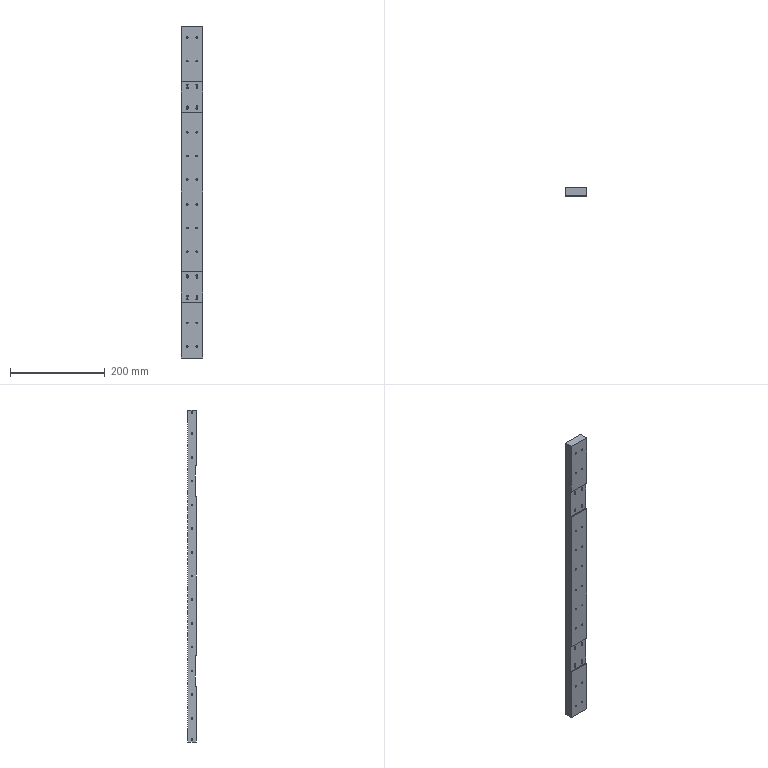Part | SolidWorks | features HoleWzd 3, Extrusion 1, ICE 1, LPattern 1 | 1 solid | 162 faces | box 45 x 18 x 700 mm | volume 549074 mm3 | cylinder 102 | cone 46 | plane 14 | commonest cylinder face diameters 3.3 x102